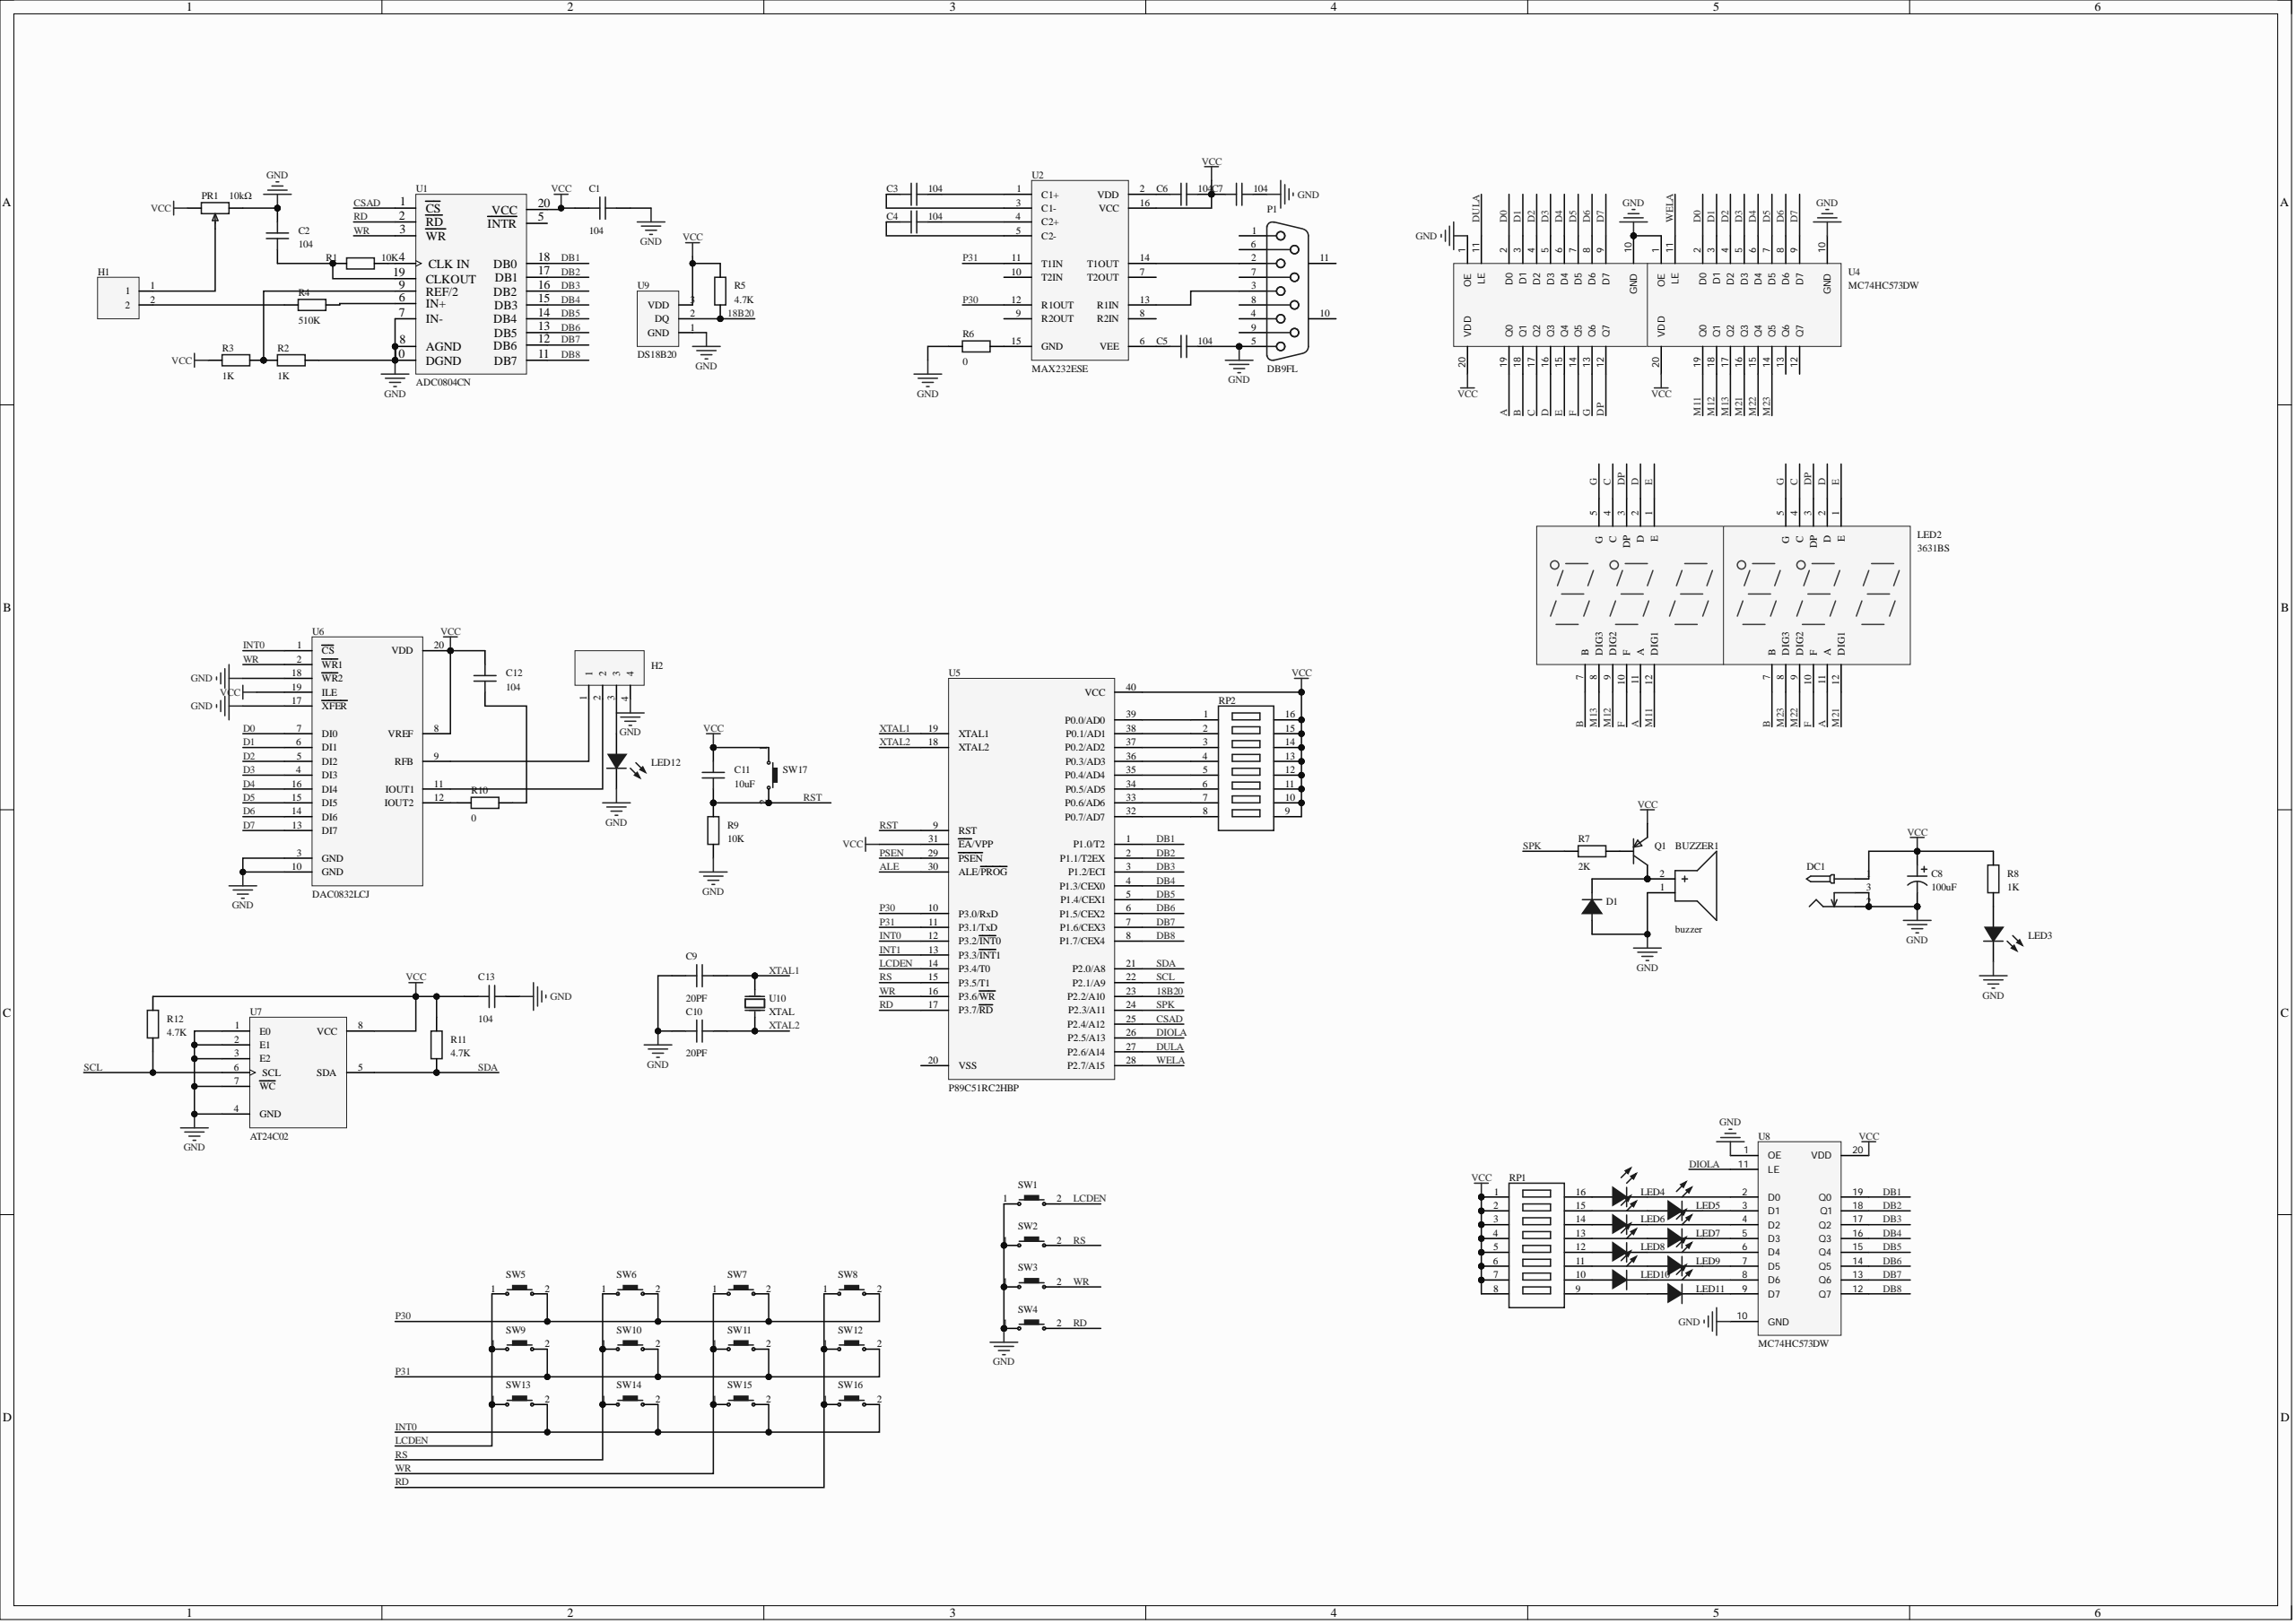Circuit board | Altium Designer | 74 parts | 97 nets
Bill of materials:
Comment,Description,Designator,Footprint,LibRef,Quantity
"buzzer","","BUZZER1","BUZ-TH_BD12.0-P6.00-D0.9-RD","buzzer","1"
"104","","C1, C2, C3, C4, C5, C6, C7, C12, C13","C0603","CAP_0603","9"
"100uF","","C8","CAP-TH_BD5.0-P2.00-D0.8-FD-10UF50VC110GL","10UF50VC110GL","1"
"20PF","","C9, C10","C0603","CAP_0603","2"
"10uF","","C11","C0603","CAP_0603","1"
"","","D1","DO_1N4007","D_1N4007A","1"
"","","DC1","DC-005_2.5","DC-005_2.5","1"
"","","H1","HDR-TH_2P-P2.54-V-M-1","HDR-M_2.54_1x2P","1"
"","","H2","HDR-TH_4P-P2.54-V-M","HDR-M_2.54_1x4P","1"
"3631BS","数码管位数:3位;发光颜色:蓝色;LED极性:共阳极;数字/字母大小(英寸):0.56;","LED1, LED2","LED-SEG-TH_11P-L37.5-W19.0-P2.54-LS15.2-BL_1","3631BS","2"
"","","LED3, LED4, LED5, LED6, LED7, LED8, LED9, LED10, LED11, LED12","LED_0603","LED_0603-B","10"
"DB9FL","","P1","DB9-TH_DB9F","DB9FL","1"
"10kΩ","","PR1","R_3296","R_3296","1"
"","","Q1","S8550P_TO-92","S8550_TO_PNP","1"
"10K","","R1, R9","R0603","Res_0603","2"
"1K","","R2, R3, R8","R0603","Res_0603","3"
"510K","","R4","R0603","Res_0603","1"
"4.7K","","R5, R11, R12","R0603","Res_0603","3"
"0","","R6, R10","R0603","Res_0603","2"
"2K","","R7","R0603","Res_0603","1"
"","","RP1, RP2","DIP-16_L20.3-W10.2-P2.54-LS7.6-BL","paizu","2"
"","","SW1, SW2, SW3, SW4, SW5, SW6, SW7, SW8, SW9, SW10, SW11, SW12, SW13, SW14, SW15, SW16, SW17","Key_SMD_3x4x2","Key_SMD_3x4x2","17"
"ADC0804CN","","U1","ADC0804CN","ADC0804CN","1"
"MAX232ESE","RS232","U2","","MAX232ESE","1"
"MC74HC573DW","","U3, U4, U8","","MC74HC573DW","3"
"P89C51RC2HBP","","U5","","P89C51RC2HBP","1"
"DAC0832LCJ","","U6","J20A","DAC0832LCJ","1"
"AT24C02","","U7","","M24C02BN6","1"
"DS18B20","","U9","TO-92-3_L4.9-W3.7-P1.27-L","DS18B20","1"
"32768/10ppm/12.5pF","","U10","osc-smd_l3.2-w1.5","32768/10ppm/12.5pF","1"
Netlist (Protel format):
[
BUZZER1
BUZ-TH_BD12.0-P6.00-D0.9-RD
buzzer



]
[
C1
C0603
104



]
[
C2
C0603
104



]
[
C3
C0603
104



]
[
C4
C0603
104



]
[
C5
C0603
104



]
[
C6
C0603
104



]
[
C7
C0603
104



]
[
C8
CAP-TH_BD5.0-P2.00-D0.8-FD-10UF50VC110GL
100uF



]
[
C9
C0603
20PF



]
[
C10
C0603
20PF



]
[
C11
C0603
10uF



]
[
C12
C0603
104



]
[
C13
C0603
104



]
[
D1
DO_1N4007




]
[
DC1
DC-005_2.5




]
[
H1
HDR-TH_2P-P2.54-V-M-1




]
[
H2
HDR-TH_4P-P2.54-V-M




]
[
LED1
LED-SEG-TH_11P-L37.5-W19.0-P2.54-LS15.2-BL_1
3631BS



]
[
LED2
LED-SEG-TH_11P-L37.5-W19.0-P2.54-LS15.2-BL_1
3631BS



]
[
LED3
LED_0603




]
[
LED4
LED_0603




]
[
LED5
LED_0603




]
[
LED6
LED_0603




]
[
LED7
LED_0603




]
[
LED8
LED_0603




]
[
LED9
LED_0603




]
[
LED10
LED_0603




]
[
LED11
LED_0603




]
[
LED12
LED_0603




]
[
P1
DB9-TH_DB9F
DB9FL



]
[
PR1
R_3296
10kΩ



]
[
Q1
S8550P_TO-92




]
[
R1
R0603
10K



]
[
R2
R0603
1K



]
[
R3
R0603
1K



]
[
R4
R0603
510K



]
[
R5
R0603
4.7K



]
[
R6
R0603
0



]
[
R7
R0603
2K



]
[
R8
R0603
1K



]
[
R9
R0603
10K



]
[
R10
R0603
0



]
[
R11
R0603
4.7K



]
[
R12
R0603
4.7K



]
[
RP1
DIP-16_L20.3-W10.2-P2.54-LS7.6-BL




]
[
RP2
DIP-16_L20.3-W10.2-P2.54-LS7.6-BL




]
[
SW1
Key_SMD_3x4x2




]
[
SW2
Key_SMD_3x4x2




]
[
SW3
Key_SMD_3x4x2




]
[
SW4
Key_SMD_3x4x2




]
[
SW5
Key_SMD_3x4x2




]
[
SW6
Key_SMD_3x4x2




]
[
SW7
Key_SMD_3x4x2




]
[
SW8
Key_SMD_3x4x2




]
[
SW9
Key_SMD_3x4x2




]
[
SW10
Key_SMD_3x4x2




]
[
SW11
Key_SMD_3x4x2




]
[
SW12
Key_SMD_3x4x2




]
[
SW13
Key_SMD_3x4x2




]
[
SW14
Key_SMD_3x4x2




]
[
SW15
Key_SMD_3x4x2




]
[
SW16
Key_SMD_3x4x2




]
[
SW17
Key_SMD_3x4x2




]
[
U1
ADC0804CN
ADC0804CN



]
[
U2

MAX232ESE



]
[
U3

MC74HC573DW



]
[
U4

MC74HC573DW



]
[
U5

P89C51RC2HBP



]
[
U6
J20A
DAC0832LCJ



]
[
U7

AT24C02



]
[
U8

MC74HC573DW



]
[
U9
TO-92-3_L4.9-W3.7-P1.27-L
DS18B20



]
[
U10
osc-smd_l3.2-w1.5
32768/10ppm/12.5pF



]
(
XTAL2
C10-2
U5-18
U10-1
)
(
XTAL1
C9-2
U5-19
U10-2
)
(
WR
SW3-2
SW7-1
SW11-1
SW15-1
U1-3
U5-16
U6-2
)
(
WELA
U4-11
U5-28
)
(
VCC
C1-1
C6-1
C7-2
C8-1
C11-2
C12-2
C13-1
DC1-1
PR1-1
Q1-1
R3-1
R5-2
R8-2
R11-2
R12-2
RP1-1
RP1-2
RP1-3
RP1-4
RP1-5
RP1-6
RP1-7
RP1-8
RP2-9
RP2-10
RP2-11
RP2-12
RP2-13
RP2-14
RP2-15
RP2-16
SW17-1
U1-20
U2-16
U3-20
U4-20
U5-31
U5-40
U6-8
U6-19
U6-20
U7-8
U8-20
U9-3
)
(
SPK
R7-1
U5-24
)
(
SDA
R11-1
U5-21
U7-5
)
(
SCL
R12-1
U5-22
U7-6
)
(
RST
C11-1
R9-2
SW17-2
U5-9
)
(
RS
SW2-2
SW6-1
SW10-1
SW14-1
U5-15
)
(
RD
SW4-2
SW8-1
SW12-1
SW16-1
U1-2
U5-17
)
(
P31
SW9-2
SW10-2
SW11-2
SW12-2
U2-11
U5-11
)
(
P30
SW5-2
SW6-2
SW7-2
SW8-2
U2-12
U5-10
)
(
NetRP2_8
RP2-8
U5-32
)
(
NetRP2_7
RP2-7
U5-33
)
(
NetRP2_6
RP2-6
U5-34
)
(
NetRP2_5
RP2-5
U5-35
)
(
NetRP2_4
RP2-4
U5-36
)
(
NetRP2_3
RP2-3
U5-37
)
(
NetRP2_2
RP2-2
U5-38
)
(
NetRP2_1
RP2-1
U5-39
)
(
NetR10_1
R10-1
U6-12
)
(
NetR6_2
R6-2
U2-15
)
(
NetR4_2
R4-2
U1-6
)
(
NetR2_1
R2-1
R3-2
U1-9
)
(
NetR1_2
R1-2
U1-4
)
(
NetQ1_2
Q1-2
R7-2
)
(
NetP1_3
P1-3
U2-13
)
(
NetP1_2
P1-2
U2-14
)
(
NetLED11_2
LED11-2
RP1-9
)
(
NetLED11_1
LED11-1
U8-9
)
(
NetLED10_2
LED10-2
RP1-10
)
(
NetLED10_1
LED10-1
U8-8
)
(
NetLED9_2
LED9-2
RP1-11
)
(
NetLED9_1
LED9-1
U8-7
)
(
NetLED8_2
LED8-2
RP1-12
)
(
NetLED8_1
LED8-1
U8-6
)
(
NetLED7_2
LED7-2
RP1-13
)
(
NetLED7_1
LED7-1
U8-5
)
(
NetLED6_2
LED6-2
RP1-14
)
(
NetLED6_1
LED6-1
U8-4
)
(
NetLED5_2
LED5-2
RP1-15
)
(
NetLED5_1
LED5-1
U8-3
)
(
NetLED4_2
LED4-2
RP1-16
)
(
NetLED4_1
LED4-1
U8-2
)
(
NetLED3_2
LED3-2
R8-1
)
(
NetH2_3
H2-3
LED12-2
)
(
NetH2_2
H2-2
U6-11
)
(
NetH2_1
H2-1
U6-9
)
(
NetH1_2
H1-2
R4-1
)
(
NetH1_1
H1-1
PR1-2
)
(
NetC12_1
C12-1
R10-2
)
(
NetC6_2
C6-2
U2-2
)
(
NetC5_2
C5-2
U2-6
)
(
NetC4_2
C4-2
U2-5
)
(
NetC4_1
C4-1
U2-4
)
(
NetC3_2
C3-2
U2-3
)
(
NetC3_1
C3-1
U2-1
)
(
NetC2_1
C2-1
R1-1
U1-19
)
(
NetBUZZER1_2
BUZZER1-2
D1-1
Q1-3
)
(
M23
LED2-8
U4-14
)
(
M22
LED2-9
U4-15
)
(
M21
LED2-12
U4-16
)
(
M13
LED1-8
U4-17
)
(
M12
LED1-9
U4-18
)
(
M11
LED1-12
U4-19
)
(
LCDEN
SW1-2
SW5-1
SW9-1
SW13-1
U5-14
)
(
INT0
SW13-2
SW14-2
SW15-2
SW16-2
U5-12
U6-1
)
(
GND
BUZZER1-1
C1-2
C2-2
C5-1
C7-1
C8-2
C9-1
C10-1
C13-2
D1-2
DC1-2
DC1-3
H2-4
LED3-1
LED12-1
P1-5
PR1-3
R2-2
R6-1
R9-1
SW1-1
SW2-1
SW3-1
SW4-1
U1-7
U1-8
U1-10
U3-1
U3-10
U4-1
U4-10
U6-3
U6-10
U6-17
U6-18
U7-1
U7-2
U7-3
U7-4
U7-7
U8-1
U8-10
U9-1
)
(
G
LED1-5
LED2-5
U3-13
)
(
F
LED1-10
LED2-10
U3-14
)
(
E
LED1-1
LED2-1
U3-15
)
(
DULA
U3-11
U5-27
)
(
DP
LED1-3
LED2-3
U3-12
)
(
DIOLA
U5-26
U8-11
)
(
DB8
U1-11
U5-8
U8-12
)
(
DB7
U1-12
U5-7
U8-13
)
(
DB6
U1-13
U5-6
U8-14
)
(
DB5
U1-14
U5-5
U8-15
)
(
DB4
U1-15
U5-4
U8-16
)
(
DB3
U1-16
U5-3
U8-17
)
(
DB2
U1-17
U5-2
U8-18
)
(
DB1
U1-18
U5-1
U8-19
)
(
D7
U3-9
U4-9
U6-13
)
(
D6
U3-8
U4-8
U6-14
)
(
D5
U3-7
U4-7
U6-15
)
(
D4
U3-6
U4-6
U6-16
)
(
D3
U3-5
U4-5
U6-4
)
(
D2
U3-4
U4-4
U6-5
)
(
D1
U3-3
U4-3
U6-6
)
(
D0
U3-2
U4-2
U6-7
)
(
D
LED1-2
LED2-2
U3-16
)
(
CSAD
U1-1
U5-25
)
(
C
LED1-4
LED2-4
U3-17
)
(
B
LED1-7
LED2-7
U3-18
)
(
A
LED1-11
LED2-11
U3-19
)
(
18B20
R5-1
U5-23
U9-2
)